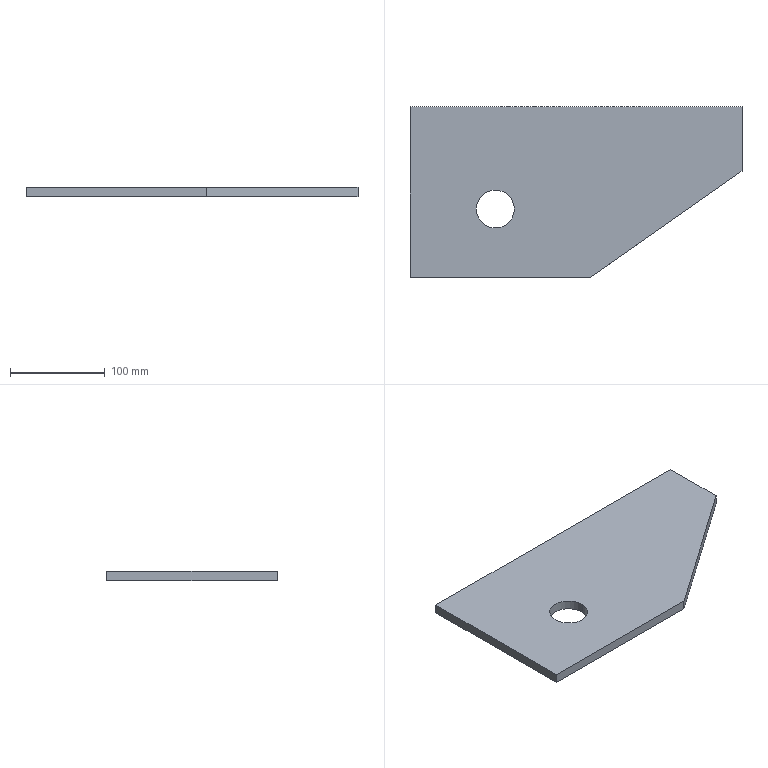Part | NX | features BREP 1, DATUM_CSYS 1, SKETCH 1 | 1 solid | 9 faces | box 350 x 180 x 10 mm | volume 527834 mm3 | plane 7 | cylinder 2 | commonest cylinder face diameters 40 x2
STEP:
#1=CARTESIAN_POINT('',(-105.,-18.,-5.));
#2=VERTEX_POINT('',#1);
#3=CARTESIAN_POINT('',(-65.,-18.,-5.));
#4=VERTEX_POINT('',#3);
#5=CARTESIAN_POINT('',(-85.,-18.,-5.));
#6=DIRECTION('',(0.,0.,1.));
#7=DIRECTION('',(1.,0.,0.));
#8=AXIS2_PLACEMENT_3D('',#5,#6,#7);
#9=CIRCLE('',#8,20.);
#10=EDGE_CURVE('',#2,#4,#9,.T.);
#11=ORIENTED_EDGE('',*,*,#10,.F.);
#12=CARTESIAN_POINT('',(-105.,-18.,5.));
#13=VERTEX_POINT('',#12);
#14=CARTESIAN_POINT('',(-105.,-18.,-5.));
#15=DIRECTION('',(0.,0.,1.));
#16=VECTOR('',#15,1000.);
#17=LINE('',#14,#16);
#18=EDGE_CURVE('',#2,#13,#17,.T.);
#19=ORIENTED_EDGE('',*,*,#18,.T.);
#20=CARTESIAN_POINT('',(-65.,-18.,5.));
#21=VERTEX_POINT('',#20);
#22=CARTESIAN_POINT('',(-85.,-18.,5.));
#23=DIRECTION('',(0.,0.,1.));
#24=DIRECTION('',(1.,0.,0.));
#25=AXIS2_PLACEMENT_3D('',#22,#23,#24);
#26=CIRCLE('',#25,20.);
#27=EDGE_CURVE('',#13,#21,#26,.T.);
#28=ORIENTED_EDGE('',*,*,#27,.T.);
#29=CARTESIAN_POINT('',(-65.,-18.,-5.));
#30=DIRECTION('',(0.,0.,1.));
#31=VECTOR('',#30,1000.);
#32=LINE('',#29,#31);
#33=EDGE_CURVE('',#4,#21,#32,.T.);
#34=ORIENTED_EDGE('',*,*,#33,.F.);
#35=EDGE_LOOP('',(#11,#19,#28,#34));
#36=FACE_BOUND('',#35,.T.);
#37=CARTESIAN_POINT('',(-85.,-18.,-5.));
#38=DIRECTION('',(0.,0.,1.));
#39=DIRECTION('',(-1.,0.,0.));
#40=AXIS2_PLACEMENT_3D('',#37,#38,#39);
#41=CYLINDRICAL_SURFACE('',#40,20.);
#42=ADVANCED_FACE('',(#36),#41,.F.);
#43=CARTESIAN_POINT('',(15.,-90.,-5.));
#44=VERTEX_POINT('',#43);
#45=CARTESIAN_POINT('',(15.,-90.,5.));
#46=VERTEX_POINT('',#45);
#47=CARTESIAN_POINT('',(15.,-90.,-497.125));
#48=DIRECTION('',(0.,0.,1.));
#49=VECTOR('',#48,1000.);
#50=LINE('',#47,#49);
#51=EDGE_CURVE('',#44,#46,#50,.T.);
#52=ORIENTED_EDGE('',*,*,#51,.T.);
#53=CARTESIAN_POINT('',(-175.,-90.,5.));
#54=VERTEX_POINT('',#53);
#55=CARTESIAN_POINT('',(-175.,-90.,5.));
#56=DIRECTION('',(1.,0.,0.));
#57=VECTOR('',#56,1000.);
#58=LINE('',#55,#57);
#59=EDGE_CURVE('',#54,#46,#58,.T.);
#60=ORIENTED_EDGE('',*,*,#59,.F.);
#61=CARTESIAN_POINT('',(-175.,-90.,-5.));
#62=VERTEX_POINT('',#61);
#63=CARTESIAN_POINT('',(-175.,-90.,5.));
#64=DIRECTION('',(0.,0.,-1.));
#65=VECTOR('',#64,1000.);
#66=LINE('',#63,#65);
#67=EDGE_CURVE('',#54,#62,#66,.T.);
#68=ORIENTED_EDGE('',*,*,#67,.T.);
#69=CARTESIAN_POINT('',(-175.,-90.,-5.));
#70=DIRECTION('',(1.,0.,0.));
#71=VECTOR('',#70,1000.);
#72=LINE('',#69,#71);
#73=EDGE_CURVE('',#62,#44,#72,.T.);
#74=ORIENTED_EDGE('',*,*,#73,.T.);
#75=EDGE_LOOP('',(#52,#60,#68,#74));
#76=FACE_BOUND('',#75,.T.);
#77=CARTESIAN_POINT('',(-175.,-90.,5.));
#78=DIRECTION('',(0.,1.,0.));
#79=DIRECTION('',(0.,0.,-1.));
#80=AXIS2_PLACEMENT_3D('',#77,#78,#79);
#81=PLANE('',#80);
#82=ADVANCED_FACE('',(#76),#81,.F.);
#83=CARTESIAN_POINT('',(175.,22.,-5.));
#84=VERTEX_POINT('',#83);
#85=CARTESIAN_POINT('',(175.,22.,5.));
#86=VERTEX_POINT('',#85);
#87=CARTESIAN_POINT('',(175.,22.,-497.125));
#88=DIRECTION('',(0.,0.,1.));
#89=VECTOR('',#88,1000.);
#90=LINE('',#87,#89);
#91=EDGE_CURVE('',#84,#86,#90,.T.);
#92=ORIENTED_EDGE('',*,*,#91,.F.);
#93=CARTESIAN_POINT('',(175.,90.,-5.));
#94=VERTEX_POINT('',#93);
#95=CARTESIAN_POINT('',(175.,90.,-5.));
#96=DIRECTION('',(0.,1.,0.));
#97=VECTOR('',#96,1000.);
#98=LINE('',#95,#97);
#99=EDGE_CURVE('',#84,#94,#98,.T.);
#100=ORIENTED_EDGE('',*,*,#99,.T.);
#101=CARTESIAN_POINT('',(175.,90.,5.));
#102=VERTEX_POINT('',#101);
#103=CARTESIAN_POINT('',(175.,90.,5.));
#104=DIRECTION('',(0.,0.,-1.));
#105=VECTOR('',#104,1000.);
#106=LINE('',#103,#105);
#107=EDGE_CURVE('',#102,#94,#106,.T.);
#108=ORIENTED_EDGE('',*,*,#107,.F.);
#109=CARTESIAN_POINT('',(175.,90.,5.));
#110=DIRECTION('',(0.,1.,0.));
#111=VECTOR('',#110,1000.);
#112=LINE('',#109,#111);
#113=EDGE_CURVE('',#86,#102,#112,.T.);
#114=ORIENTED_EDGE('',*,*,#113,.F.);
#115=EDGE_LOOP('',(#92,#100,#108,#114));
#116=FACE_BOUND('',#115,.T.);
#117=CARTESIAN_POINT('',(175.,90.,5.));
#118=DIRECTION('',(-1.,0.,0.));
#119=DIRECTION('',(0.,1.,0.));
#120=AXIS2_PLACEMENT_3D('',#117,#118,#119);
#121=PLANE('',#120);
#122=ADVANCED_FACE('',(#116),#121,.F.);
#123=CARTESIAN_POINT('',(-85.,-18.,5.));
#124=DIRECTION('',(0.,0.,1.));
#125=DIRECTION('',(1.,0.,0.));
#126=AXIS2_PLACEMENT_3D('',#123,#124,#125);
#127=CIRCLE('',#126,20.);
#128=EDGE_CURVE('',#21,#13,#127,.T.);
#129=ORIENTED_EDGE('',*,*,#128,.F.);
#130=ORIENTED_EDGE('',*,*,#27,.F.);
#131=EDGE_LOOP('',(#129,#130));
#132=FACE_BOUND('',#131,.T.);
#133=ORIENTED_EDGE('',*,*,#59,.T.);
#134=CARTESIAN_POINT('',(-112.517,-179.262,5.));
#135=DIRECTION('',(0.8192,0.5735,0.));
#136=VECTOR('',#135,1000.);
#137=LINE('',#134,#136);
#138=EDGE_CURVE('',#46,#86,#137,.T.);
#139=ORIENTED_EDGE('',*,*,#138,.T.);
#140=ORIENTED_EDGE('',*,*,#113,.T.);
#141=CARTESIAN_POINT('',(-175.,90.,5.));
#142=VERTEX_POINT('',#141);
#143=CARTESIAN_POINT('',(-175.,90.,5.));
#144=DIRECTION('',(-1.,0.,0.));
#145=VECTOR('',#144,1000.);
#146=LINE('',#143,#145);
#147=EDGE_CURVE('',#102,#142,#146,.T.);
#148=ORIENTED_EDGE('',*,*,#147,.T.);
#149=CARTESIAN_POINT('',(-175.,90.,5.));
#150=DIRECTION('',(0.,-1.,0.));
#151=VECTOR('',#150,1000.);
#152=LINE('',#149,#151);
#153=EDGE_CURVE('',#142,#54,#152,.T.);
#154=ORIENTED_EDGE('',*,*,#153,.T.);
#155=EDGE_LOOP('',(#133,#139,#140,#148,#154));
#156=FACE_BOUND('',#155,.T.);
#157=CARTESIAN_POINT('',(-175.,-90.,5.));
#158=DIRECTION('',(0.,0.,1.));
#159=DIRECTION('',(-1.,0.,0.));
#160=AXIS2_PLACEMENT_3D('',#157,#158,#159);
#161=PLANE('',#160);
#162=ADVANCED_FACE('',(#132,#156),#161,.T.);
#163=CARTESIAN_POINT('',(-85.,-18.,-5.));
#164=DIRECTION('',(0.,0.,1.));
#165=DIRECTION('',(1.,0.,0.));
#166=AXIS2_PLACEMENT_3D('',#163,#164,#165);
#167=CIRCLE('',#166,20.);
#168=EDGE_CURVE('',#4,#2,#167,.T.);
#169=ORIENTED_EDGE('',*,*,#168,.T.);
#170=ORIENTED_EDGE('',*,*,#10,.T.);
#171=EDGE_LOOP('',(#169,#170));
#172=FACE_BOUND('',#171,.T.);
#173=CARTESIAN_POINT('',(-112.517,-179.262,-5.));
#174=DIRECTION('',(0.8192,0.5735,0.));
#175=VECTOR('',#174,1000.);
#176=LINE('',#173,#175);
#177=EDGE_CURVE('',#44,#84,#176,.T.);
#178=ORIENTED_EDGE('',*,*,#177,.F.);
#179=ORIENTED_EDGE('',*,*,#73,.F.);
#180=CARTESIAN_POINT('',(-175.,90.,-5.));
#181=VERTEX_POINT('',#180);
#182=CARTESIAN_POINT('',(-175.,90.,-5.));
#183=DIRECTION('',(0.,-1.,0.));
#184=VECTOR('',#183,1000.);
#185=LINE('',#182,#184);
#186=EDGE_CURVE('',#181,#62,#185,.T.);
#187=ORIENTED_EDGE('',*,*,#186,.F.);
#188=CARTESIAN_POINT('',(-175.,90.,-5.));
#189=DIRECTION('',(-1.,0.,0.));
#190=VECTOR('',#189,1000.);
#191=LINE('',#188,#190);
#192=EDGE_CURVE('',#94,#181,#191,.T.);
#193=ORIENTED_EDGE('',*,*,#192,.F.);
#194=ORIENTED_EDGE('',*,*,#99,.F.);
#195=EDGE_LOOP('',(#178,#179,#187,#193,#194));
#196=FACE_BOUND('',#195,.T.);
#197=CARTESIAN_POINT('',(-175.,-90.,-5.));
#198=DIRECTION('',(0.,0.,1.));
#199=DIRECTION('',(-1.,0.,0.));
#200=AXIS2_PLACEMENT_3D('',#197,#198,#199);
#201=PLANE('',#200);
#202=ADVANCED_FACE('',(#172,#196),#201,.F.);
#203=ORIENTED_EDGE('',*,*,#186,.T.);
#204=ORIENTED_EDGE('',*,*,#67,.F.);
#205=ORIENTED_EDGE('',*,*,#153,.F.);
#206=CARTESIAN_POINT('',(-175.,90.,5.));
#207=DIRECTION('',(0.,0.,-1.));
#208=VECTOR('',#207,1000.);
#209=LINE('',#206,#208);
#210=EDGE_CURVE('',#142,#181,#209,.T.);
#211=ORIENTED_EDGE('',*,*,#210,.T.);
#212=EDGE_LOOP('',(#203,#204,#205,#211));
#213=FACE_BOUND('',#212,.T.);
#214=CARTESIAN_POINT('',(-175.,90.,5.));
#215=DIRECTION('',(1.,0.,0.));
#216=DIRECTION('',(0.,-1.,0.));
#217=AXIS2_PLACEMENT_3D('',#214,#215,#216);
#218=PLANE('',#217);
#219=ADVANCED_FACE('',(#213),#218,.F.);
#220=ORIENTED_EDGE('',*,*,#192,.T.);
#221=ORIENTED_EDGE('',*,*,#210,.F.);
#222=ORIENTED_EDGE('',*,*,#147,.F.);
#223=ORIENTED_EDGE('',*,*,#107,.T.);
#224=EDGE_LOOP('',(#220,#221,#222,#223));
#225=FACE_BOUND('',#224,.T.);
#226=CARTESIAN_POINT('',(-175.,90.,5.));
#227=DIRECTION('',(0.,-1.,0.));
#228=DIRECTION('',(0.,0.,1.));
#229=AXIS2_PLACEMENT_3D('',#226,#227,#228);
#230=PLANE('',#229);
#231=ADVANCED_FACE('',(#225),#230,.F.);
#232=ORIENTED_EDGE('',*,*,#138,.F.);
#233=ORIENTED_EDGE('',*,*,#51,.F.);
#234=ORIENTED_EDGE('',*,*,#177,.T.);
#235=ORIENTED_EDGE('',*,*,#91,.T.);
#236=EDGE_LOOP('',(#232,#233,#234,#235));
#237=FACE_BOUND('',#236,.T.);
#238=CARTESIAN_POINT('',(15.,-90.,-497.125));
#239=DIRECTION('',(0.5735,-0.8192,0.));
#240=DIRECTION('',(-0.8192,-0.5735,0.));
#241=AXIS2_PLACEMENT_3D('',#238,#239,#240);
#242=PLANE('',#241);
#243=ADVANCED_FACE('',(#237),#242,.T.);
#244=ORIENTED_EDGE('',*,*,#18,.F.);
#245=ORIENTED_EDGE('',*,*,#168,.F.);
#246=ORIENTED_EDGE('',*,*,#33,.T.);
#247=ORIENTED_EDGE('',*,*,#128,.T.);
#248=EDGE_LOOP('',(#244,#245,#246,#247));
#249=FACE_BOUND('',#248,.T.);
#250=CARTESIAN_POINT('',(-85.,-18.,-5.));
#251=DIRECTION('',(0.,0.,1.));
#252=DIRECTION('',(-1.,0.,0.));
#253=AXIS2_PLACEMENT_3D('',#250,#251,#252);
#254=CYLINDRICAL_SURFACE('',#253,20.);
#255=ADVANCED_FACE('',(#249),#254,.F.);
#256=CLOSED_SHELL('',(#42,#82,#122,#162,#202,#219,#231,#243,#255));
#257=MANIFOLD_SOLID_BREP('',#256);
#258=(LENGTH_UNIT()NAMED_UNIT(*)SI_UNIT(.MILLI.,.METRE.));
#259=UNCERTAINTY_MEASURE_WITH_UNIT(LENGTH_MEASURE(0.00001),#258,'','');
#260=(NAMED_UNIT(*)PLANE_ANGLE_UNIT()SI_UNIT($,.RADIAN.));
#261=(NAMED_UNIT(*)SI_UNIT($,.STERADIAN.)SOLID_ANGLE_UNIT());
#262=(GEOMETRIC_REPRESENTATION_CONTEXT(3)GLOBAL_UNCERTAINTY_ASSIGNED_CONTEXT((#259))GLOBAL_UNIT_ASSIGNED_CONTEXT((#258,#260,#261))REPRESENTATION_CONTEXT('',''));
#263=ADVANCED_BREP_SHAPE_REPRESENTATION('',(#257),#262);